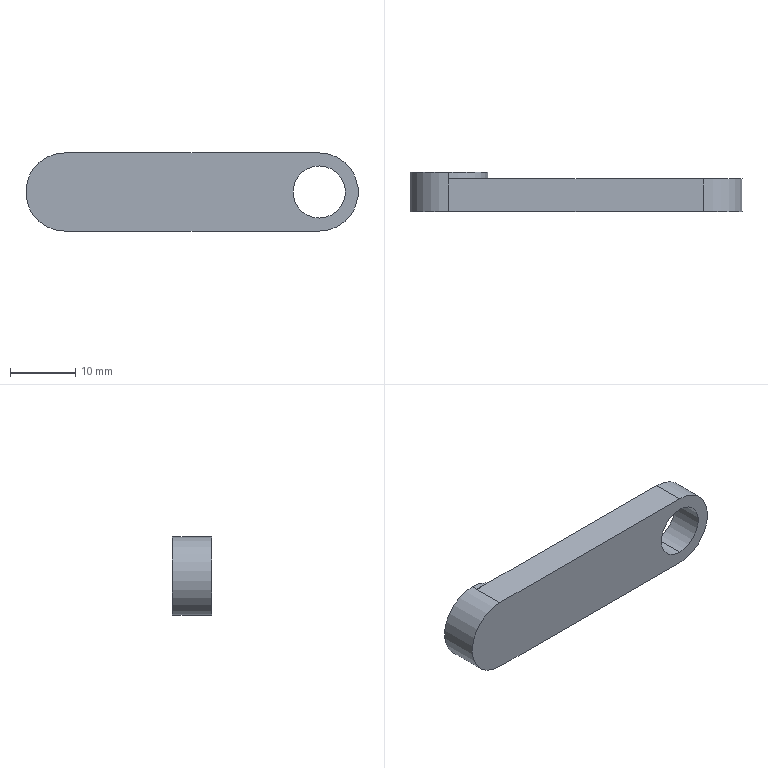Part | STEP file | 444_Default | 1 solid | 10 faces | box 51 x 6 x 12 mm | volume 2767 mm3 | cylinder 5 | plane 5 | commonest cylinder face diameters 12 x3 8 x2
STEP:
#1=CARTESIAN_POINT('',(0.,0.,0.));
#2=DIRECTION('',(0.,0.,1.));
#3=DIRECTION('',(1.,0.,0.));
#4=AXIS2_PLACEMENT_3D('',#1,#2,#3);
#5=CARTESIAN_POINT('',(19.5,0.,4.));
#6=VERTEX_POINT('',#5);
#7=CARTESIAN_POINT('',(19.5,5.,4.));
#8=VERTEX_POINT('',#7);
#9=CARTESIAN_POINT('',(19.5,-0.000025,4.));
#10=DIRECTION('',(0.,1.,0.));
#11=VECTOR('',#10,1.);
#12=LINE('',#9,#11);
#13=CARTESIAN_POINT('',(19.5,-0.000025,0.));
#14=DIRECTION('',(0.,1.,0.));
#15=DIRECTION('',(0.,0.,1.));
#16=AXIS2_PLACEMENT_3D('',#13,#14,#15);
#17=CYLINDRICAL_SURFACE('',#16,4.);
#18=CARTESIAN_POINT('',(6.283,0.));
#19=DIRECTION('',(0.,1.));
#20=VECTOR('',#19,1.);
#21=LINE('',#18,#20);
#22=(GEOMETRIC_REPRESENTATION_CONTEXT(2)PARAMETRIC_REPRESENTATION_CONTEXT()REPRESENTATION_CONTEXT('',''));
#23=DEFINITIONAL_REPRESENTATION('',(#21),#22);
#24=PCURVE('',#17,#23);
#25=CARTESIAN_POINT('',(19.5,-0.000025,0.));
#26=DIRECTION('',(0.,1.,0.));
#27=DIRECTION('',(0.,0.,1.));
#28=AXIS2_PLACEMENT_3D('',#25,#26,#27);
#29=CYLINDRICAL_SURFACE('',#28,4.);
#30=CARTESIAN_POINT('',(0.,0.));
#31=DIRECTION('',(0.,1.));
#32=VECTOR('',#31,1.);
#33=LINE('',#30,#32);
#34=(GEOMETRIC_REPRESENTATION_CONTEXT(2)PARAMETRIC_REPRESENTATION_CONTEXT()REPRESENTATION_CONTEXT('',''));
#35=DEFINITIONAL_REPRESENTATION('',(#33),#34);
#36=PCURVE('',#29,#35);
#37=SURFACE_CURVE('',#12,(#24,#36),.PCURVE_S1.);
#38=EDGE_CURVE('',#6,#8,#37,.T.);
#39=ORIENTED_EDGE('',*,*,#38,.T.);
#40=CARTESIAN_POINT('',(19.5,5.,-4.));
#41=VERTEX_POINT('',#40);
#42=CARTESIAN_POINT('',(19.5,5.,0.));
#43=DIRECTION('',(0.,1.,0.));
#44=DIRECTION('',(0.,0.,1.));
#45=AXIS2_PLACEMENT_3D('',#42,#43,#44);
#46=CIRCLE('',#45,4.);
#47=CARTESIAN_POINT('',(0.,5.));
#48=DIRECTION('',(1.,0.));
#49=VECTOR('',#48,1.);
#50=LINE('',#47,#49);
#51=(GEOMETRIC_REPRESENTATION_CONTEXT(2)PARAMETRIC_REPRESENTATION_CONTEXT()REPRESENTATION_CONTEXT('',''));
#52=DEFINITIONAL_REPRESENTATION('',(#50),#51);
#53=PCURVE('',#17,#52);
#54=CARTESIAN_POINT('',(19.5,5.,0.));
#55=DIRECTION('',(0.,1.,0.));
#56=DIRECTION('',(0.,0.,1.));
#57=AXIS2_PLACEMENT_3D('',#54,#55,#56);
#58=PLANE('',#57);
#59=CARTESIAN_POINT('',(0.,0.));
#60=DIRECTION('',(1.,0.));
#61=AXIS2_PLACEMENT_2D('',#59,#60);
#62=CIRCLE('',#61,4.);
#63=(GEOMETRIC_REPRESENTATION_CONTEXT(2)PARAMETRIC_REPRESENTATION_CONTEXT()REPRESENTATION_CONTEXT('',''));
#64=DEFINITIONAL_REPRESENTATION('',(#62),#63);
#65=PCURVE('',#58,#64);
#66=SURFACE_CURVE('',#46,(#53,#65),.PCURVE_S1.);
#67=EDGE_CURVE('',#41,#8,#66,.T.);
#68=ORIENTED_EDGE('',*,*,#67,.F.);
#69=CARTESIAN_POINT('',(19.5,0.,-4.));
#70=VERTEX_POINT('',#69);
#71=CARTESIAN_POINT('',(19.5,-0.000025,-4.));
#72=DIRECTION('',(0.,1.,0.));
#73=VECTOR('',#72,1.);
#74=LINE('',#71,#73);
#75=CARTESIAN_POINT('',(3.142,0.));
#76=DIRECTION('',(0.,1.));
#77=VECTOR('',#76,1.);
#78=LINE('',#75,#77);
#79=(GEOMETRIC_REPRESENTATION_CONTEXT(2)PARAMETRIC_REPRESENTATION_CONTEXT()REPRESENTATION_CONTEXT('',''));
#80=DEFINITIONAL_REPRESENTATION('',(#78),#79);
#81=PCURVE('',#17,#80);
#82=CARTESIAN_POINT('',(3.142,0.));
#83=DIRECTION('',(0.,1.));
#84=VECTOR('',#83,1.);
#85=LINE('',#82,#84);
#86=(GEOMETRIC_REPRESENTATION_CONTEXT(2)PARAMETRIC_REPRESENTATION_CONTEXT()REPRESENTATION_CONTEXT('',''));
#87=DEFINITIONAL_REPRESENTATION('',(#85),#86);
#88=PCURVE('',#29,#87);
#89=SURFACE_CURVE('',#74,(#81,#88),.PCURVE_S1.);
#90=EDGE_CURVE('',#70,#41,#89,.T.);
#91=ORIENTED_EDGE('',*,*,#90,.F.);
#92=CARTESIAN_POINT('',(19.5,0.,0.));
#93=DIRECTION('',(0.,1.,0.));
#94=DIRECTION('',(0.,0.,1.));
#95=AXIS2_PLACEMENT_3D('',#92,#93,#94);
#96=CIRCLE('',#95,4.);
#97=CARTESIAN_POINT('',(0.,0.000025));
#98=DIRECTION('',(1.,0.));
#99=VECTOR('',#98,1.);
#100=LINE('',#97,#99);
#101=(GEOMETRIC_REPRESENTATION_CONTEXT(2)PARAMETRIC_REPRESENTATION_CONTEXT()REPRESENTATION_CONTEXT('',''));
#102=DEFINITIONAL_REPRESENTATION('',(#100),#101);
#103=PCURVE('',#17,#102);
#104=CARTESIAN_POINT('',(19.5,0.,0.));
#105=DIRECTION('',(0.,1.,0.));
#106=DIRECTION('',(0.,0.,1.));
#107=AXIS2_PLACEMENT_3D('',#104,#105,#106);
#108=PLANE('',#107);
#109=CARTESIAN_POINT('',(0.,0.));
#110=DIRECTION('',(1.,0.));
#111=AXIS2_PLACEMENT_2D('',#109,#110);
#112=CIRCLE('',#111,4.);
#113=(GEOMETRIC_REPRESENTATION_CONTEXT(2)PARAMETRIC_REPRESENTATION_CONTEXT()REPRESENTATION_CONTEXT('',''));
#114=DEFINITIONAL_REPRESENTATION('',(#112),#113);
#115=PCURVE('',#108,#114);
#116=SURFACE_CURVE('',#96,(#103,#115),.PCURVE_S1.);
#117=EDGE_CURVE('',#70,#6,#116,.T.);
#118=ORIENTED_EDGE('',*,*,#117,.T.);
#119=EDGE_LOOP('',(#39,#68,#91,#118));
#120=FACE_BOUND('',#119,.F.);
#121=ADVANCED_FACE('',(#120),#17,.F.);
#122=CARTESIAN_POINT('',(-19.5,6.,6.));
#123=VERTEX_POINT('',#122);
#124=CARTESIAN_POINT('',(-19.5,6.,-6.));
#125=VERTEX_POINT('',#124);
#126=CARTESIAN_POINT('',(-19.5,6.,0.));
#127=DIRECTION('',(0.,1.,0.));
#128=DIRECTION('',(0.,0.,1.));
#129=AXIS2_PLACEMENT_3D('',#126,#127,#128);
#130=CIRCLE('',#129,6.);
#131=CARTESIAN_POINT('',(-19.5,5.,0.));
#132=DIRECTION('',(0.,-1.,0.));
#133=DIRECTION('',(0.,0.,-1.));
#134=AXIS2_PLACEMENT_3D('',#131,#132,#133);
#135=CYLINDRICAL_SURFACE('',#134,6.);
#136=CARTESIAN_POINT('',(3.142,-1.));
#137=DIRECTION('',(-1.,0.));
#138=VECTOR('',#137,1.);
#139=LINE('',#136,#138);
#140=(GEOMETRIC_REPRESENTATION_CONTEXT(2)PARAMETRIC_REPRESENTATION_CONTEXT()REPRESENTATION_CONTEXT('',''));
#141=DEFINITIONAL_REPRESENTATION('',(#139),#140);
#142=PCURVE('',#135,#141);
#143=CARTESIAN_POINT('',(-19.5,6.,0.));
#144=DIRECTION('',(0.,1.,0.));
#145=DIRECTION('',(0.,0.,1.));
#146=AXIS2_PLACEMENT_3D('',#143,#144,#145);
#147=PLANE('',#146);
#148=CARTESIAN_POINT('',(0.,0.));
#149=DIRECTION('',(1.,0.));
#150=AXIS2_PLACEMENT_2D('',#148,#149);
#151=CIRCLE('',#150,6.);
#152=(GEOMETRIC_REPRESENTATION_CONTEXT(2)PARAMETRIC_REPRESENTATION_CONTEXT()REPRESENTATION_CONTEXT('',''));
#153=DEFINITIONAL_REPRESENTATION('',(#151),#152);
#154=PCURVE('',#147,#153);
#155=SURFACE_CURVE('',#130,(#142,#154),.PCURVE_S1.);
#156=EDGE_CURVE('',#123,#125,#155,.T.);
#157=ORIENTED_EDGE('',*,*,#156,.F.);
#158=CARTESIAN_POINT('',(-19.5,5.,6.));
#159=VERTEX_POINT('',#158);
#160=CARTESIAN_POINT('',(-19.5,5.,6.));
#161=DIRECTION('',(0.,-1.,0.));
#162=VECTOR('',#161,1.);
#163=LINE('',#160,#162);
#164=CARTESIAN_POINT('',(3.142,0.));
#165=DIRECTION('',(0.,1.));
#166=VECTOR('',#165,1.);
#167=LINE('',#164,#166);
#168=(GEOMETRIC_REPRESENTATION_CONTEXT(2)PARAMETRIC_REPRESENTATION_CONTEXT()REPRESENTATION_CONTEXT('',''));
#169=DEFINITIONAL_REPRESENTATION('',(#167),#168);
#170=PCURVE('',#135,#169);
#171=CARTESIAN_POINT('',(-19.5,5.,0.));
#172=DIRECTION('',(0.,-1.,0.));
#173=DIRECTION('',(0.,0.,-1.));
#174=AXIS2_PLACEMENT_3D('',#171,#172,#173);
#175=CYLINDRICAL_SURFACE('',#174,6.);
#176=CARTESIAN_POINT('',(3.142,0.));
#177=DIRECTION('',(0.,1.));
#178=VECTOR('',#177,1.);
#179=LINE('',#176,#178);
#180=(GEOMETRIC_REPRESENTATION_CONTEXT(2)PARAMETRIC_REPRESENTATION_CONTEXT()REPRESENTATION_CONTEXT('',''));
#181=DEFINITIONAL_REPRESENTATION('',(#179),#180);
#182=PCURVE('',#175,#181);
#183=SURFACE_CURVE('',#163,(#170,#182),.PCURVE_S1.);
#184=EDGE_CURVE('',#123,#159,#183,.T.);
#185=ORIENTED_EDGE('',*,*,#184,.T.);
#186=CARTESIAN_POINT('',(-19.5,5.,-6.));
#187=VERTEX_POINT('',#186);
#188=CARTESIAN_POINT('',(-19.5,5.,0.));
#189=DIRECTION('',(0.,1.,0.));
#190=DIRECTION('',(0.,0.,1.));
#191=AXIS2_PLACEMENT_3D('',#188,#189,#190);
#192=CIRCLE('',#191,6.);
#193=CARTESIAN_POINT('',(3.142,0.));
#194=DIRECTION('',(-1.,0.));
#195=VECTOR('',#194,1.);
#196=LINE('',#193,#195);
#197=(GEOMETRIC_REPRESENTATION_CONTEXT(2)PARAMETRIC_REPRESENTATION_CONTEXT()REPRESENTATION_CONTEXT('',''));
#198=DEFINITIONAL_REPRESENTATION('',(#196),#197);
#199=PCURVE('',#135,#198);
#200=CARTESIAN_POINT('',(0.,-39.));
#201=DIRECTION('',(1.,0.));
#202=AXIS2_PLACEMENT_2D('',#200,#201);
#203=CIRCLE('',#202,6.);
#204=(GEOMETRIC_REPRESENTATION_CONTEXT(2)PARAMETRIC_REPRESENTATION_CONTEXT()REPRESENTATION_CONTEXT('',''));
#205=DEFINITIONAL_REPRESENTATION('',(#203),#204);
#206=PCURVE('',#58,#205);
#207=SURFACE_CURVE('',#192,(#199,#206),.PCURVE_S1.);
#208=EDGE_CURVE('',#159,#187,#207,.T.);
#209=ORIENTED_EDGE('',*,*,#208,.T.);
#210=CARTESIAN_POINT('',(-19.5,5.,-6.));
#211=DIRECTION('',(0.,-1.,0.));
#212=VECTOR('',#211,1.);
#213=LINE('',#210,#212);
#214=CARTESIAN_POINT('',(0.,0.));
#215=DIRECTION('',(0.,1.));
#216=VECTOR('',#215,1.);
#217=LINE('',#214,#216);
#218=(GEOMETRIC_REPRESENTATION_CONTEXT(2)PARAMETRIC_REPRESENTATION_CONTEXT()REPRESENTATION_CONTEXT('',''));
#219=DEFINITIONAL_REPRESENTATION('',(#217),#218);
#220=PCURVE('',#135,#219);
#221=CARTESIAN_POINT('',(6.283,0.));
#222=DIRECTION('',(0.,1.));
#223=VECTOR('',#222,1.);
#224=LINE('',#221,#223);
#225=(GEOMETRIC_REPRESENTATION_CONTEXT(2)PARAMETRIC_REPRESENTATION_CONTEXT()REPRESENTATION_CONTEXT('',''));
#226=DEFINITIONAL_REPRESENTATION('',(#224),#225);
#227=PCURVE('',#175,#226);
#228=SURFACE_CURVE('',#213,(#220,#227),.PCURVE_S1.);
#229=EDGE_CURVE('',#125,#187,#228,.T.);
#230=ORIENTED_EDGE('',*,*,#229,.F.);
#231=EDGE_LOOP('',(#157,#185,#209,#230));
#232=FACE_BOUND('',#231,.T.);
#233=ADVANCED_FACE('',(#232),#135,.T.);
#234=CARTESIAN_POINT('',(19.5,0.,6.));
#235=VERTEX_POINT('',#234);
#236=CARTESIAN_POINT('',(19.5,0.,-6.));
#237=VERTEX_POINT('',#236);
#238=CARTESIAN_POINT('',(19.5,0.,0.));
#239=DIRECTION('',(0.,1.,0.));
#240=DIRECTION('',(0.,0.,1.));
#241=AXIS2_PLACEMENT_3D('',#238,#239,#240);
#242=CIRCLE('',#241,6.);
#243=CARTESIAN_POINT('',(19.5,5.,0.));
#244=DIRECTION('',(0.,-1.,0.));
#245=DIRECTION('',(0.,0.,-1.));
#246=AXIS2_PLACEMENT_3D('',#243,#244,#245);
#247=CYLINDRICAL_SURFACE('',#246,6.);
#248=CARTESIAN_POINT('',(3.142,5.));
#249=DIRECTION('',(-1.,0.));
#250=VECTOR('',#249,1.);
#251=LINE('',#248,#250);
#252=(GEOMETRIC_REPRESENTATION_CONTEXT(2)PARAMETRIC_REPRESENTATION_CONTEXT()REPRESENTATION_CONTEXT('',''));
#253=DEFINITIONAL_REPRESENTATION('',(#251),#252);
#254=PCURVE('',#247,#253);
#255=CARTESIAN_POINT('',(0.,0.));
#256=DIRECTION('',(1.,0.));
#257=AXIS2_PLACEMENT_2D('',#255,#256);
#258=CIRCLE('',#257,6.);
#259=(GEOMETRIC_REPRESENTATION_CONTEXT(2)PARAMETRIC_REPRESENTATION_CONTEXT()REPRESENTATION_CONTEXT('',''));
#260=DEFINITIONAL_REPRESENTATION('',(#258),#259);
#261=PCURVE('',#108,#260);
#262=SURFACE_CURVE('',#242,(#254,#261),.PCURVE_S1.);
#263=EDGE_CURVE('',#235,#237,#262,.T.);
#264=ORIENTED_EDGE('',*,*,#263,.T.);
#265=CARTESIAN_POINT('',(19.5,5.,-6.));
#266=VERTEX_POINT('',#265);
#267=CARTESIAN_POINT('',(19.5,5.,-6.));
#268=DIRECTION('',(0.,-1.,0.));
#269=VECTOR('',#268,1.);
#270=LINE('',#267,#269);
#271=CARTESIAN_POINT('',(0.,0.));
#272=DIRECTION('',(0.,1.));
#273=VECTOR('',#272,1.);
#274=LINE('',#271,#273);
#275=(GEOMETRIC_REPRESENTATION_CONTEXT(2)PARAMETRIC_REPRESENTATION_CONTEXT()REPRESENTATION_CONTEXT('',''));
#276=DEFINITIONAL_REPRESENTATION('',(#274),#275);
#277=PCURVE('',#247,#276);
#278=CARTESIAN_POINT('',(19.5,5.,-6.));
#279=DIRECTION('',(0.,0.,1.));
#280=DIRECTION('',(1.,0.,0.));
#281=AXIS2_PLACEMENT_3D('',#278,#279,#280);
#282=PLANE('',#281);
#283=CARTESIAN_POINT('',(0.,0.));
#284=DIRECTION('',(0.,-1.));
#285=VECTOR('',#284,1.);
#286=LINE('',#283,#285);
#287=(GEOMETRIC_REPRESENTATION_CONTEXT(2)PARAMETRIC_REPRESENTATION_CONTEXT()REPRESENTATION_CONTEXT('',''));
#288=DEFINITIONAL_REPRESENTATION('',(#286),#287);
#289=PCURVE('',#282,#288);
#290=SURFACE_CURVE('',#270,(#277,#289),.PCURVE_S1.);
#291=EDGE_CURVE('',#266,#237,#290,.T.);
#292=ORIENTED_EDGE('',*,*,#291,.F.);
#293=CARTESIAN_POINT('',(19.5,5.,6.));
#294=VERTEX_POINT('',#293);
#295=CARTESIAN_POINT('',(19.5,5.,0.));
#296=DIRECTION('',(0.,1.,0.));
#297=DIRECTION('',(0.,0.,1.));
#298=AXIS2_PLACEMENT_3D('',#295,#296,#297);
#299=CIRCLE('',#298,6.);
#300=CARTESIAN_POINT('',(3.142,0.));
#301=DIRECTION('',(-1.,0.));
#302=VECTOR('',#301,1.);
#303=LINE('',#300,#302);
#304=(GEOMETRIC_REPRESENTATION_CONTEXT(2)PARAMETRIC_REPRESENTATION_CONTEXT()REPRESENTATION_CONTEXT('',''));
#305=DEFINITIONAL_REPRESENTATION('',(#303),#304);
#306=PCURVE('',#247,#305);
#307=CARTESIAN_POINT('',(0.,0.));
#308=DIRECTION('',(1.,0.));
#309=AXIS2_PLACEMENT_2D('',#307,#308);
#310=CIRCLE('',#309,6.);
#311=(GEOMETRIC_REPRESENTATION_CONTEXT(2)PARAMETRIC_REPRESENTATION_CONTEXT()REPRESENTATION_CONTEXT('',''));
#312=DEFINITIONAL_REPRESENTATION('',(#310),#311);
#313=PCURVE('',#58,#312);
#314=SURFACE_CURVE('',#299,(#306,#313),.PCURVE_S1.);
#315=EDGE_CURVE('',#294,#266,#314,.T.);
#316=ORIENTED_EDGE('',*,*,#315,.F.);
#317=CARTESIAN_POINT('',(19.5,5.,6.));
#318=DIRECTION('',(0.,-1.,0.));
#319=VECTOR('',#318,1.);
#320=LINE('',#317,#319);
#321=CARTESIAN_POINT('',(3.142,0.));
#322=DIRECTION('',(0.,1.));
#323=VECTOR('',#322,1.);
#324=LINE('',#321,#323);
#325=(GEOMETRIC_REPRESENTATION_CONTEXT(2)PARAMETRIC_REPRESENTATION_CONTEXT()REPRESENTATION_CONTEXT('',''));
#326=DEFINITIONAL_REPRESENTATION('',(#324),#325);
#327=PCURVE('',#247,#326);
#328=CARTESIAN_POINT('',(19.5,5.,6.));
#329=DIRECTION('',(0.,0.,-1.));
#330=DIRECTION('',(-1.,0.,0.));
#331=AXIS2_PLACEMENT_3D('',#328,#329,#330);
#332=PLANE('',#331);
#333=CARTESIAN_POINT('',(0.,0.));
#334=DIRECTION('',(0.,-1.));
#335=VECTOR('',#334,1.);
#336=LINE('',#333,#335);
#337=(GEOMETRIC_REPRESENTATION_CONTEXT(2)PARAMETRIC_REPRESENTATION_CONTEXT()REPRESENTATION_CONTEXT('',''));
#338=DEFINITIONAL_REPRESENTATION('',(#336),#337);
#339=PCURVE('',#332,#338);
#340=SURFACE_CURVE('',#320,(#327,#339),.PCURVE_S1.);
#341=EDGE_CURVE('',#294,#235,#340,.T.);
#342=ORIENTED_EDGE('',*,*,#341,.T.);
#343=EDGE_LOOP('',(#264,#292,#316,#342));
#344=FACE_BOUND('',#343,.T.);
#345=ADVANCED_FACE('',(#344),#247,.T.);
#346=CARTESIAN_POINT('',(-19.5,0.,-6.));
#347=VERTEX_POINT('',#346);
#348=CARTESIAN_POINT('',(19.5,0.,-6.));
#349=DIRECTION('',(-1.,0.,0.));
#350=VECTOR('',#349,1.);
#351=LINE('',#348,#350);
#352=CARTESIAN_POINT('',(0.,-5.));
#353=DIRECTION('',(-1.,0.));
#354=VECTOR('',#353,1.);
#355=LINE('',#352,#354);
#356=(GEOMETRIC_REPRESENTATION_CONTEXT(2)PARAMETRIC_REPRESENTATION_CONTEXT()REPRESENTATION_CONTEXT('',''));
#357=DEFINITIONAL_REPRESENTATION('',(#355),#356);
#358=PCURVE('',#282,#357);
#359=CARTESIAN_POINT('',(-6.,0.));
#360=DIRECTION('',(0.,-1.));
#361=VECTOR('',#360,1.);
#362=LINE('',#359,#361);
#363=(GEOMETRIC_REPRESENTATION_CONTEXT(2)PARAMETRIC_REPRESENTATION_CONTEXT()REPRESENTATION_CONTEXT('',''));
#364=DEFINITIONAL_REPRESENTATION('',(#362),#363);
#365=PCURVE('',#108,#364);
#366=SURFACE_CURVE('',#351,(#358,#365),.PCURVE_S1.);
#367=EDGE_CURVE('',#237,#347,#366,.T.);
#368=ORIENTED_EDGE('',*,*,#367,.T.);
#369=CARTESIAN_POINT('',(-19.5,5.,-6.));
#370=DIRECTION('',(0.,-1.,0.));
#371=VECTOR('',#370,1.);
#372=LINE('',#369,#371);
#373=CARTESIAN_POINT('',(-39.,0.));
#374=DIRECTION('',(0.,-1.));
#375=VECTOR('',#374,1.);
#376=LINE('',#373,#375);
#377=(GEOMETRIC_REPRESENTATION_CONTEXT(2)PARAMETRIC_REPRESENTATION_CONTEXT()REPRESENTATION_CONTEXT('',''));
#378=DEFINITIONAL_REPRESENTATION('',(#376),#377);
#379=PCURVE('',#282,#378);
#380=CARTESIAN_POINT('',(6.283,0.));
#381=DIRECTION('',(0.,1.));
#382=VECTOR('',#381,1.);
#383=LINE('',#380,#382);
#384=(GEOMETRIC_REPRESENTATION_CONTEXT(2)PARAMETRIC_REPRESENTATION_CONTEXT()REPRESENTATION_CONTEXT('',''));
#385=DEFINITIONAL_REPRESENTATION('',(#383),#384);
#386=PCURVE('',#175,#385);
#387=SURFACE_CURVE('',#372,(#379,#386),.PCURVE_S1.);
#388=EDGE_CURVE('',#187,#347,#387,.T.);
#389=ORIENTED_EDGE('',*,*,#388,.F.);
#390=CARTESIAN_POINT('',(19.5,5.,-6.));
#391=DIRECTION('',(-1.,0.,0.));
#392=VECTOR('',#391,1.);
#393=LINE('',#390,#392);
#394=CARTESIAN_POINT('',(0.,0.));
#395=DIRECTION('',(-1.,0.));
#396=VECTOR('',#395,1.);
#397=LINE('',#394,#396);
#398=(GEOMETRIC_REPRESENTATION_CONTEXT(2)PARAMETRIC_REPRESENTATION_CONTEXT()REPRESENTATION_CONTEXT('',''));
#399=DEFINITIONAL_REPRESENTATION('',(#397),#398);
#400=PCURVE('',#282,#399);
#401=CARTESIAN_POINT('',(-6.,0.));
#402=DIRECTION('',(0.,-1.));
#403=VECTOR('',#402,1.);
#404=LINE('',#401,#403);
#405=(GEOMETRIC_REPRESENTATION_CONTEXT(2)PARAMETRIC_REPRESENTATION_CONTEXT()REPRESENTATION_CONTEXT('',''));
#406=DEFINITIONAL_REPRESENTATION('',(#404),#405);
#407=PCURVE('',#58,#406);
#408=SURFACE_CURVE('',#393,(#400,#407),.PCURVE_S1.);
#409=EDGE_CURVE('',#266,#187,#408,.T.);
#410=ORIENTED_EDGE('',*,*,#409,.F.);
#411=ORIENTED_EDGE('',*,*,#291,.T.);
#412=EDGE_LOOP('',(#368,#389,#410,#411));
#413=FACE_BOUND('',#412,.T.);
#414=ADVANCED_FACE('',(#413),#282,.F.);
#415=ORIENTED_EDGE('',*,*,#184,.F.);
#416=CARTESIAN_POINT('',(-19.5,6.,0.));
#417=DIRECTION('',(0.,1.,0.));
#418=DIRECTION('',(0.,0.,1.));
#419=AXIS2_PLACEMENT_3D('',#416,#417,#418);
#420=CIRCLE('',#419,6.);
#421=CARTESIAN_POINT('',(9.425,-1.));
#422=DIRECTION('',(-1.,0.));
#423=VECTOR('',#422,1.);
#424=LINE('',#421,#423);
#425=(GEOMETRIC_REPRESENTATION_CONTEXT(2)PARAMETRIC_REPRESENTATION_CONTEXT()REPRESENTATION_CONTEXT('',''));
#426=DEFINITIONAL_REPRESENTATION('',(#424),#425);
#427=PCURVE('',#175,#426);
#428=CARTESIAN_POINT('',(0.,0.));
#429=DIRECTION('',(1.,0.));
#430=AXIS2_PLACEMENT_2D('',#428,#429);
#431=CIRCLE('',#430,6.);
#432=(GEOMETRIC_REPRESENTATION_CONTEXT(2)PARAMETRIC_REPRESENTATION_CONTEXT()REPRESENTATION_CONTEXT('',''));
#433=DEFINITIONAL_REPRESENTATION('',(#431),#432);
#434=PCURVE('',#147,#433);
#435=SURFACE_CURVE('',#420,(#427,#434),.PCURVE_S1.);
#436=EDGE_CURVE('',#125,#123,#435,.T.);
#437=ORIENTED_EDGE('',*,*,#436,.F.);
#438=ORIENTED_EDGE('',*,*,#229,.T.);
#439=ORIENTED_EDGE('',*,*,#388,.T.);
#440=CARTESIAN_POINT('',(-19.5,0.,6.));
#441=VERTEX_POINT('',#440);
#442=CARTESIAN_POINT('',(-19.5,0.,0.));
#443=DIRECTION('',(0.,1.,0.));
#444=DIRECTION('',(0.,0.,1.));
#445=AXIS2_PLACEMENT_3D('',#442,#443,#444);
#446=CIRCLE('',#445,6.);
#447=CARTESIAN_POINT('',(9.425,5.));
#448=DIRECTION('',(-1.,0.));
#449=VECTOR('',#448,1.);
#450=LINE('',#447,#449);
#451=(GEOMETRIC_REPRESENTATION_CONTEXT(2)PARAMETRIC_REPRESENTATION_CONTEXT()REPRESENTATION_CONTEXT('',''));
#452=DEFINITIONAL_REPRESENTATION('',(#450),#451);
#453=PCURVE('',#175,#452);
#454=CARTESIAN_POINT('',(0.,-39.));
#455=DIRECTION('',(1.,0.));
#456=AXIS2_PLACEMENT_2D('',#454,#455);
#457=CIRCLE('',#456,6.);
#458=(GEOMETRIC_REPRESENTATION_CONTEXT(2)PARAMETRIC_REPRESENTATION_CONTEXT()REPRESENTATION_CONTEXT('',''));
#459=DEFINITIONAL_REPRESENTATION('',(#457),#458);
#460=PCURVE('',#108,#459);
#461=SURFACE_CURVE('',#446,(#453,#460),.PCURVE_S1.);
#462=EDGE_CURVE('',#347,#441,#461,.T.);
#463=ORIENTED_EDGE('',*,*,#462,.T.);
#464=CARTESIAN_POINT('',(-19.5,5.,6.));
#465=DIRECTION('',(0.,-1.,0.));
#466=VECTOR('',#465,1.);
#467=LINE('',#464,#466);
#468=CARTESIAN_POINT('',(3.142,0.));
#469=DIRECTION('',(0.,1.));
#470=VECTOR('',#469,1.);
#471=LINE('',#468,#470);
#472=(GEOMETRIC_REPRESENTATION_CONTEXT(2)PARAMETRIC_REPRESENTATION_CONTEXT()REPRESENTATION_CONTEXT('',''));
#473=DEFINITIONAL_REPRESENTATION('',(#471),#472);
#474=PCURVE('',#175,#473);
#475=CARTESIAN_POINT('',(39.,0.));
#476=DIRECTION('',(0.,-1.));
#477=VECTOR('',#476,1.);
#478=LINE('',#475,#477);
#479=(GEOMETRIC_REPRESENTATION_CONTEXT(2)PARAMETRIC_REPRESENTATION_CONTEXT()REPRESENTATION_CONTEXT('',''));
#480=DEFINITIONAL_REPRESENTATION('',(#478),#479);
#481=PCURVE('',#332,#480);
#482=SURFACE_CURVE('',#467,(#474,#481),.PCURVE_S1.);
#483=EDGE_CURVE('',#159,#441,#482,.T.);
#484=ORIENTED_EDGE('',*,*,#483,.F.);
#485=EDGE_LOOP('',(#415,#437,#438,#439,#463,#484));
#486=FACE_BOUND('',#485,.T.);
#487=ADVANCED_FACE('',(#486),#175,.T.);
#488=CARTESIAN_POINT('',(19.5,0.,6.));
#489=DIRECTION('',(1.,0.,0.));
#490=VECTOR('',#489,1.);
#491=LINE('',#488,#490);
#492=CARTESIAN_POINT('',(0.,-5.));
#493=DIRECTION('',(-1.,0.));
#494=VECTOR('',#493,1.);
#495=LINE('',#492,#494);
#496=(GEOMETRIC_REPRESENTATION_CONTEXT(2)PARAMETRIC_REPRESENTATION_CONTEXT()REPRESENTATION_CONTEXT('',''));
#497=DEFINITIONAL_REPRESENTATION('',(#495),#496);
#498=PCURVE('',#332,#497);
#499=CARTESIAN_POINT('',(6.,0.));
#500=DIRECTION('',(0.,1.));
#501=VECTOR('',#500,1.);
#502=LINE('',#499,#501);
#503=(GEOMETRIC_REPRESENTATION_CONTEXT(2)PARAMETRIC_REPRESENTATION_CONTEXT()REPRESENTATION_CONTEXT('',''));
#504=DEFINITIONAL_REPRESENTATION('',(#502),#503);
#505=PCURVE('',#108,#504);
#506=SURFACE_CURVE('',#491,(#498,#505),.PCURVE_S1.);
#507=EDGE_CURVE('',#441,#235,#506,.T.);
#508=ORIENTED_EDGE('',*,*,#507,.T.);
#509=ORIENTED_EDGE('',*,*,#341,.F.);
#510=CARTESIAN_POINT('',(19.5,5.,6.));
#511=DIRECTION('',(1.,0.,0.));
#512=VECTOR('',#511,1.);
#513=LINE('',#510,#512);
#514=CARTESIAN_POINT('',(0.,0.));
#515=DIRECTION('',(-1.,0.));
#516=VECTOR('',#515,1.);
#517=LINE('',#514,#516);
#518=(GEOMETRIC_REPRESENTATION_CONTEXT(2)PARAMETRIC_REPRESENTATION_CONTEXT()REPRESENTATION_CONTEXT('',''));
#519=DEFINITIONAL_REPRESENTATION('',(#517),#518);
#520=PCURVE('',#332,#519);
#521=CARTESIAN_POINT('',(6.,0.));
#522=DIRECTION('',(0.,1.));
#523=VECTOR('',#522,1.);
#524=LINE('',#521,#523);
#525=(GEOMETRIC_REPRESENTATION_CONTEXT(2)PARAMETRIC_REPRESENTATION_CONTEXT()REPRESENTATION_CONTEXT('',''));
#526=DEFINITIONAL_REPRESENTATION('',(#524),#525);
#527=PCURVE('',#58,#526);
#528=SURFACE_CURVE('',#513,(#520,#527),.PCURVE_S1.);
#529=EDGE_CURVE('',#159,#294,#528,.T.);
#530=ORIENTED_EDGE('',*,*,#529,.F.);
#531=ORIENTED_EDGE('',*,*,#483,.T.);
#532=EDGE_LOOP('',(#508,#509,#530,#531));
#533=FACE_BOUND('',#532,.T.);
#534=ADVANCED_FACE('',(#533),#332,.F.);
#535=CARTESIAN_POINT('',(19.5,5.,0.));
#536=DIRECTION('',(0.,1.,0.));
#537=DIRECTION('',(0.,0.,1.));
#538=AXIS2_PLACEMENT_3D('',#535,#536,#537);
#539=CIRCLE('',#538,4.);
#540=CARTESIAN_POINT('',(0.,0.));
#541=DIRECTION('',(1.,0.));
#542=AXIS2_PLACEMENT_2D('',#540,#541);
#543=CIRCLE('',#542,4.);
#544=(GEOMETRIC_REPRESENTATION_CONTEXT(2)PARAMETRIC_REPRESENTATION_CONTEXT()REPRESENTATION_CONTEXT('',''));
#545=DEFINITIONAL_REPRESENTATION('',(#543),#544);
#546=PCURVE('',#58,#545);
#547=CARTESIAN_POINT('',(0.,5.));
#548=DIRECTION('',(1.,0.));
#549=VECTOR('',#548,1.);
#550=LINE('',#547,#549);
#551=(GEOMETRIC_REPRESENTATION_CONTEXT(2)PARAMETRIC_REPRESENTATION_CONTEXT()REPRESENTATION_CONTEXT('',''));
#552=DEFINITIONAL_REPRESENTATION('',(#550),#551);
#553=PCURVE('',#29,#552);
#554=SURFACE_CURVE('',#539,(#546,#553),.PCURVE_S1.);
#555=EDGE_CURVE('',#8,#41,#554,.T.);
#556=ORIENTED_EDGE('',*,*,#555,.F.);
#557=ORIENTED_EDGE('',*,*,#67,.F.);
#558=EDGE_LOOP('',(#556,#557));
#559=FACE_BOUND('',#558,.T.);
#560=ORIENTED_EDGE('',*,*,#208,.F.);
#561=ORIENTED_EDGE('',*,*,#529,.T.);
#562=ORIENTED_EDGE('',*,*,#315,.T.);
#563=ORIENTED_EDGE('',*,*,#409,.T.);
#564=EDGE_LOOP('',(#560,#561,#562,#563));
#565=FACE_BOUND('',#564,.T.);
#566=ADVANCED_FACE('',(#559,#565),#58,.T.);
#567=CARTESIAN_POINT('',(19.5,0.,0.));
#568=DIRECTION('',(0.,1.,0.));
#569=DIRECTION('',(0.,0.,1.));
#570=AXIS2_PLACEMENT_3D('',#567,#568,#569);
#571=CIRCLE('',#570,4.);
#572=CARTESIAN_POINT('',(0.,0.));
#573=DIRECTION('',(1.,0.));
#574=AXIS2_PLACEMENT_2D('',#572,#573);
#575=CIRCLE('',#574,4.);
#576=(GEOMETRIC_REPRESENTATION_CONTEXT(2)PARAMETRIC_REPRESENTATION_CONTEXT()REPRESENTATION_CONTEXT('',''));
#577=DEFINITIONAL_REPRESENTATION('',(#575),#576);
#578=PCURVE('',#108,#577);
#579=CARTESIAN_POINT('',(0.,0.000025));
#580=DIRECTION('',(1.,0.));
#581=VECTOR('',#580,1.);
#582=LINE('',#579,#581);
#583=(GEOMETRIC_REPRESENTATION_CONTEXT(2)PARAMETRIC_REPRESENTATION_CONTEXT()REPRESENTATION_CONTEXT('',''));
#584=DEFINITIONAL_REPRESENTATION('',(#582),#583);
#585=PCURVE('',#29,#584);
#586=SURFACE_CURVE('',#571,(#578,#585),.PCURVE_S1.);
#587=EDGE_CURVE('',#6,#70,#586,.T.);
#588=ORIENTED_EDGE('',*,*,#587,.T.);
#589=ORIENTED_EDGE('',*,*,#117,.T.);
#590=EDGE_LOOP('',(#588,#589));
#591=FACE_BOUND('',#590,.T.);
#592=ORIENTED_EDGE('',*,*,#263,.F.);
#593=ORIENTED_EDGE('',*,*,#507,.F.);
#594=ORIENTED_EDGE('',*,*,#462,.F.);
#595=ORIENTED_EDGE('',*,*,#367,.F.);
#596=EDGE_LOOP('',(#592,#593,#594,#595));
#597=FACE_BOUND('',#596,.T.);
#598=ADVANCED_FACE('',(#591,#597),#108,.F.);
#599=ORIENTED_EDGE('',*,*,#436,.T.);
#600=ORIENTED_EDGE('',*,*,#156,.T.);
#601=EDGE_LOOP('',(#599,#600));
#602=FACE_BOUND('',#601,.T.);
#603=ADVANCED_FACE('',(#602),#147,.T.);
#604=ORIENTED_EDGE('',*,*,#555,.F.);
#605=ORIENTED_EDGE('',*,*,#38,.F.);
#606=ORIENTED_EDGE('',*,*,#587,.T.);
#607=ORIENTED_EDGE('',*,*,#90,.T.);
#608=EDGE_LOOP('',(#604,#605,#606,#607));
#609=FACE_BOUND('',#608,.F.);
#610=ADVANCED_FACE('',(#609),#29,.F.);
#611=CLOSED_SHELL('',(#121,#233,#345,#414,#487,#534,#566,#598,#603,#610));
#612=MANIFOLD_SOLID_BREP('',#611);
#613=(LENGTH_UNIT()NAMED_UNIT(*)SI_UNIT(.MILLI.,.METRE.));
#614=UNCERTAINTY_MEASURE_WITH_UNIT(LENGTH_MEASURE(0.0000001),#613,'','');
#615=(NAMED_UNIT(*)PLANE_ANGLE_UNIT()SI_UNIT($,.RADIAN.));
#616=(NAMED_UNIT(*)SI_UNIT($,.STERADIAN.)SOLID_ANGLE_UNIT());
#617=(GEOMETRIC_REPRESENTATION_CONTEXT(3)GLOBAL_UNCERTAINTY_ASSIGNED_CONTEXT((#614))GLOBAL_UNIT_ASSIGNED_CONTEXT((#613,#615,#616))REPRESENTATION_CONTEXT('',''));
#618=ADVANCED_BREP_SHAPE_REPRESENTATION('',(#4,#612),#617);